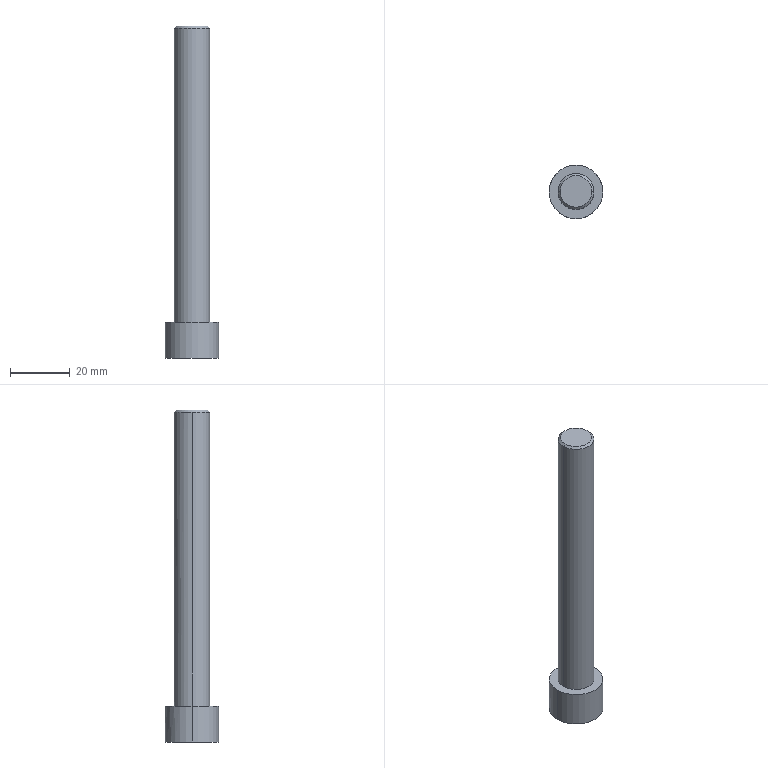Part | Creo | 1 solid | 16 faces | box 18 x 18 x 111 mm | volume 13555 mm3 | plane 10 | cylinder 4 | cone 2 | commonest cylinder face diameters 12 x2 18 x2
STEP:
#1=CARTESIAN_POINT('',(0.,0.,0.));
#2=DIRECTION('',(0.,0.,1.));
#3=DIRECTION('',(1.,0.,0.));
#4=AXIS2_PLACEMENT_3D('',#1,#2,#3);
#5=CARTESIAN_POINT('',(432.101,252.373,-117.152));
#6=VERTEX_POINT('',#5);
#7=CARTESIAN_POINT('',(420.101,252.373,-117.152));
#8=VERTEX_POINT('',#7);
#9=CARTESIAN_POINT('',(426.101,252.373,-117.152));
#10=DIRECTION('',(0.,0.,1.));
#11=DIRECTION('',(1.,0.,0.));
#12=AXIS2_PLACEMENT_3D('',#9,#10,#11);
#13=CIRCLE('',#12,6.);
#14=EDGE_CURVE('',#6,#8,#13,.T.);
#15=ORIENTED_EDGE('',*,*,#14,.T.);
#16=CARTESIAN_POINT('',(420.101,252.373,-215.441));
#17=VERTEX_POINT('',#16);
#18=CARTESIAN_POINT('',(420.101,252.373,-215.441));
#19=DIRECTION('',(0.,0.,1.));
#20=VECTOR('',#19,98.29);
#21=LINE('',#18,#20);
#22=EDGE_CURVE('',#17,#8,#21,.T.);
#23=ORIENTED_EDGE('',*,*,#22,.F.);
#24=CARTESIAN_POINT('',(426.101,258.373,-215.441));
#25=VERTEX_POINT('',#24);
#26=CARTESIAN_POINT('',(426.101,252.373,-215.441));
#27=DIRECTION('',(0.,0.,-1.));
#28=DIRECTION('',(-1.,0.,0.));
#29=AXIS2_PLACEMENT_3D('',#26,#27,#28);
#30=CIRCLE('',#29,6.);
#31=EDGE_CURVE('',#17,#25,#30,.T.);
#32=ORIENTED_EDGE('',*,*,#31,.T.);
#33=CARTESIAN_POINT('',(432.101,252.373,-215.441));
#34=VERTEX_POINT('',#33);
#35=CARTESIAN_POINT('',(426.101,252.373,-215.441));
#36=DIRECTION('',(0.,0.,-1.));
#37=DIRECTION('',(0.,1.,0.));
#38=AXIS2_PLACEMENT_3D('',#35,#36,#37);
#39=CIRCLE('',#38,6.);
#40=EDGE_CURVE('',#25,#34,#39,.T.);
#41=ORIENTED_EDGE('',*,*,#40,.T.);
#42=CARTESIAN_POINT('',(432.101,252.373,-215.441));
#43=DIRECTION('',(0.,0.,1.));
#44=VECTOR('',#43,98.29);
#45=LINE('',#42,#44);
#46=EDGE_CURVE('',#34,#6,#45,.T.);
#47=ORIENTED_EDGE('',*,*,#46,.T.);
#48=EDGE_LOOP('',(#15,#23,#32,#41,#47));
#49=FACE_OUTER_BOUND('',#48,.F.);
#50=CARTESIAN_POINT('',(426.101,252.373,-215.441));
#51=DIRECTION('',(0.,0.,1.));
#52=DIRECTION('',(1.,0.,0.));
#53=AXIS2_PLACEMENT_3D('',#50,#51,#52);
#54=CYLINDRICAL_SURFACE('',#53,6.);
#55=ADVANCED_FACE('',(#49),#54,.T.);
#56=CARTESIAN_POINT('',(426.101,257.662,-116.441));
#57=VERTEX_POINT('',#56);
#58=CARTESIAN_POINT('',(420.811,252.373,-116.441));
#59=VERTEX_POINT('',#58);
#60=CARTESIAN_POINT('',(426.101,252.373,-116.441));
#61=DIRECTION('',(0.,0.,1.));
#62=DIRECTION('',(0.,1.,0.));
#63=AXIS2_PLACEMENT_3D('',#60,#61,#62);
#64=CIRCLE('',#63,5.29);
#65=EDGE_CURVE('',#57,#59,#64,.T.);
#66=ORIENTED_EDGE('',*,*,#65,.T.);
#67=CARTESIAN_POINT('',(420.811,252.373,-116.441));
#68=DIRECTION('',(-0.7071,0.,-0.7071));
#69=VECTOR('',#68,1.005);
#70=LINE('',#67,#69);
#71=EDGE_CURVE('',#59,#8,#70,.T.);
#72=ORIENTED_EDGE('',*,*,#71,.T.);
#73=ORIENTED_EDGE('',*,*,#14,.F.);
#74=CARTESIAN_POINT('',(431.39,252.373,-116.441));
#75=VERTEX_POINT('',#74);
#76=CARTESIAN_POINT('',(431.39,252.373,-116.441));
#77=DIRECTION('',(0.7071,0.,-0.7071));
#78=VECTOR('',#77,1.005);
#79=LINE('',#76,#78);
#80=EDGE_CURVE('',#75,#6,#79,.T.);
#81=ORIENTED_EDGE('',*,*,#80,.F.);
#82=CARTESIAN_POINT('',(426.101,252.373,-116.441));
#83=DIRECTION('',(0.,0.,1.));
#84=DIRECTION('',(1.,0.,0.));
#85=AXIS2_PLACEMENT_3D('',#82,#83,#84);
#86=CIRCLE('',#85,5.29);
#87=EDGE_CURVE('',#75,#57,#86,.T.);
#88=ORIENTED_EDGE('',*,*,#87,.T.);
#89=EDGE_LOOP('',(#66,#72,#73,#81,#88));
#90=FACE_OUTER_BOUND('',#89,.F.);
#91=CARTESIAN_POINT('',(426.101,252.373,-116.797));
#92=DIRECTION('',(0.,0.,-1.));
#93=DIRECTION('',(-1.,0.,0.));
#94=AXIS2_PLACEMENT_3D('',#91,#92,#93);
#95=CONICAL_SURFACE('',#94,5.645,45.);
#96=ADVANCED_FACE('',(#90),#95,.T.);
#97=CARTESIAN_POINT('',(426.101,247.083,-116.441));
#98=VERTEX_POINT('',#97);
#99=CARTESIAN_POINT('',(426.101,252.373,-116.441));
#100=DIRECTION('',(0.,0.,1.));
#101=DIRECTION('',(0.,-1.,0.));
#102=AXIS2_PLACEMENT_3D('',#99,#100,#101);
#103=CIRCLE('',#102,5.29);
#104=EDGE_CURVE('',#98,#75,#103,.T.);
#105=ORIENTED_EDGE('',*,*,#104,.F.);
#106=CARTESIAN_POINT('',(426.101,252.373,-116.441));
#107=DIRECTION('',(0.,0.,1.));
#108=DIRECTION('',(-1.,0.,0.));
#109=AXIS2_PLACEMENT_3D('',#106,#107,#108);
#110=CIRCLE('',#109,5.29);
#111=EDGE_CURVE('',#59,#98,#110,.T.);
#112=ORIENTED_EDGE('',*,*,#111,.F.);
#113=ORIENTED_EDGE('',*,*,#65,.F.);
#114=ORIENTED_EDGE('',*,*,#87,.F.);
#115=EDGE_LOOP('',(#105,#112,#113,#114));
#116=FACE_OUTER_BOUND('',#115,.F.);
#117=CARTESIAN_POINT('',(426.101,252.373,-116.441));
#118=DIRECTION('',(0.,0.,-1.));
#119=DIRECTION('',(-1.,0.,0.));
#120=AXIS2_PLACEMENT_3D('',#117,#118,#119);
#121=PLANE('',#120);
#122=ADVANCED_FACE('',(#116),#121,.F.);
#123=ORIENTED_EDGE('',*,*,#111,.T.);
#124=ORIENTED_EDGE('',*,*,#104,.T.);
#125=ORIENTED_EDGE('',*,*,#80,.T.);
#126=CARTESIAN_POINT('',(426.101,246.373,-117.152));
#127=VERTEX_POINT('',#126);
#128=CARTESIAN_POINT('',(426.101,252.373,-117.152));
#129=DIRECTION('',(0.,0.,1.));
#130=DIRECTION('',(0.,-1.,0.));
#131=AXIS2_PLACEMENT_3D('',#128,#129,#130);
#132=CIRCLE('',#131,6.);
#133=EDGE_CURVE('',#127,#6,#132,.T.);
#134=ORIENTED_EDGE('',*,*,#133,.F.);
#135=CARTESIAN_POINT('',(426.101,252.373,-117.152));
#136=DIRECTION('',(0.,0.,1.));
#137=DIRECTION('',(-1.,0.,0.));
#138=AXIS2_PLACEMENT_3D('',#135,#136,#137);
#139=CIRCLE('',#138,6.);
#140=EDGE_CURVE('',#8,#127,#139,.T.);
#141=ORIENTED_EDGE('',*,*,#140,.F.);
#142=ORIENTED_EDGE('',*,*,#71,.F.);
#143=EDGE_LOOP('',(#123,#124,#125,#134,#141,#142));
#144=FACE_OUTER_BOUND('',#143,.F.);
#145=CARTESIAN_POINT('',(426.101,252.373,-116.797));
#146=DIRECTION('',(0.,0.,-1.));
#147=DIRECTION('',(-1.,0.,0.));
#148=AXIS2_PLACEMENT_3D('',#145,#146,#147);
#149=CONICAL_SURFACE('',#148,5.645,45.);
#150=ADVANCED_FACE('',(#144),#149,.T.);
#151=ORIENTED_EDGE('',*,*,#140,.T.);
#152=ORIENTED_EDGE('',*,*,#133,.T.);
#153=ORIENTED_EDGE('',*,*,#46,.F.);
#154=CARTESIAN_POINT('',(426.101,246.373,-215.441));
#155=VERTEX_POINT('',#154);
#156=CARTESIAN_POINT('',(426.101,252.373,-215.441));
#157=DIRECTION('',(0.,0.,-1.));
#158=DIRECTION('',(1.,0.,0.));
#159=AXIS2_PLACEMENT_3D('',#156,#157,#158);
#160=CIRCLE('',#159,6.);
#161=EDGE_CURVE('',#34,#155,#160,.T.);
#162=ORIENTED_EDGE('',*,*,#161,.T.);
#163=CARTESIAN_POINT('',(426.101,252.373,-215.441));
#164=DIRECTION('',(0.,0.,-1.));
#165=DIRECTION('',(0.,-1.,0.));
#166=AXIS2_PLACEMENT_3D('',#163,#164,#165);
#167=CIRCLE('',#166,6.);
#168=EDGE_CURVE('',#155,#17,#167,.T.);
#169=ORIENTED_EDGE('',*,*,#168,.T.);
#170=ORIENTED_EDGE('',*,*,#22,.T.);
#171=EDGE_LOOP('',(#151,#152,#153,#162,#169,#170));
#172=FACE_OUTER_BOUND('',#171,.F.);
#173=CARTESIAN_POINT('',(426.101,252.373,-215.441));
#174=DIRECTION('',(0.,0.,1.));
#175=DIRECTION('',(1.,0.,0.));
#176=AXIS2_PLACEMENT_3D('',#173,#174,#175);
#177=CYLINDRICAL_SURFACE('',#176,6.);
#178=ADVANCED_FACE('',(#172),#177,.T.);
#179=CARTESIAN_POINT('',(426.101,243.373,-215.441));
#180=VERTEX_POINT('',#179);
#181=CARTESIAN_POINT('',(435.101,252.373,-215.441));
#182=VERTEX_POINT('',#181);
#183=CARTESIAN_POINT('',(426.101,252.373,-215.441));
#184=DIRECTION('',(0.,0.,1.));
#185=DIRECTION('',(0.,-1.,0.));
#186=AXIS2_PLACEMENT_3D('',#183,#184,#185);
#187=CIRCLE('',#186,9.);
#188=EDGE_CURVE('',#180,#182,#187,.T.);
#189=ORIENTED_EDGE('',*,*,#188,.F.);
#190=CARTESIAN_POINT('',(417.101,252.373,-215.441));
#191=VERTEX_POINT('',#190);
#192=CARTESIAN_POINT('',(426.101,252.373,-215.441));
#193=DIRECTION('',(0.,0.,1.));
#194=DIRECTION('',(-1.,0.,0.));
#195=AXIS2_PLACEMENT_3D('',#192,#193,#194);
#196=CIRCLE('',#195,9.);
#197=EDGE_CURVE('',#191,#180,#196,.T.);
#198=ORIENTED_EDGE('',*,*,#197,.F.);
#199=CARTESIAN_POINT('',(426.101,252.373,-215.441));
#200=DIRECTION('',(0.,0.,1.));
#201=DIRECTION('',(1.,0.,0.));
#202=AXIS2_PLACEMENT_3D('',#199,#200,#201);
#203=CIRCLE('',#202,9.);
#204=EDGE_CURVE('',#182,#191,#203,.T.);
#205=ORIENTED_EDGE('',*,*,#204,.F.);
#206=EDGE_LOOP('',(#189,#198,#205));
#207=FACE_OUTER_BOUND('',#206,.F.);
#208=ORIENTED_EDGE('',*,*,#168,.F.);
#209=ORIENTED_EDGE('',*,*,#161,.F.);
#210=ORIENTED_EDGE('',*,*,#40,.F.);
#211=ORIENTED_EDGE('',*,*,#31,.F.);
#212=EDGE_LOOP('',(#208,#209,#210,#211));
#213=FACE_BOUND('',#212,.F.);
#214=CARTESIAN_POINT('',(426.101,252.373,-215.441));
#215=DIRECTION('',(0.,0.,1.));
#216=DIRECTION('',(1.,0.,0.));
#217=AXIS2_PLACEMENT_3D('',#214,#215,#216);
#218=PLANE('',#217);
#219=ADVANCED_FACE('',(#207,#213),#218,.T.);
#220=CARTESIAN_POINT('',(435.101,252.373,-227.441));
#221=VERTEX_POINT('',#220);
#222=CARTESIAN_POINT('',(426.101,243.373,-227.441));
#223=VERTEX_POINT('',#222);
#224=CARTESIAN_POINT('',(426.101,252.373,-227.441));
#225=DIRECTION('',(0.,0.,-1.));
#226=DIRECTION('',(1.,0.,0.));
#227=AXIS2_PLACEMENT_3D('',#224,#225,#226);
#228=CIRCLE('',#227,9.);
#229=EDGE_CURVE('',#221,#223,#228,.T.);
#230=ORIENTED_EDGE('',*,*,#229,.T.);
#231=CARTESIAN_POINT('',(417.101,252.373,-227.441));
#232=VERTEX_POINT('',#231);
#233=CARTESIAN_POINT('',(426.101,252.373,-227.441));
#234=DIRECTION('',(0.,0.,-1.));
#235=DIRECTION('',(0.,-1.,0.));
#236=AXIS2_PLACEMENT_3D('',#233,#234,#235);
#237=CIRCLE('',#236,9.);
#238=EDGE_CURVE('',#223,#232,#237,.T.);
#239=ORIENTED_EDGE('',*,*,#238,.T.);
#240=CARTESIAN_POINT('',(417.101,252.373,-215.441));
#241=DIRECTION('',(0.,0.,-1.));
#242=VECTOR('',#241,12.);
#243=LINE('',#240,#242);
#244=EDGE_CURVE('',#191,#232,#243,.T.);
#245=ORIENTED_EDGE('',*,*,#244,.F.);
#246=ORIENTED_EDGE('',*,*,#197,.T.);
#247=ORIENTED_EDGE('',*,*,#188,.T.);
#248=CARTESIAN_POINT('',(435.101,252.373,-215.441));
#249=DIRECTION('',(0.,0.,-1.));
#250=VECTOR('',#249,12.);
#251=LINE('',#248,#250);
#252=EDGE_CURVE('',#182,#221,#251,.T.);
#253=ORIENTED_EDGE('',*,*,#252,.T.);
#254=EDGE_LOOP('',(#230,#239,#245,#246,#247,#253));
#255=FACE_OUTER_BOUND('',#254,.F.);
#256=CARTESIAN_POINT('',(426.101,252.373,-215.441));
#257=DIRECTION('',(0.,0.,-1.));
#258=DIRECTION('',(-1.,0.,0.));
#259=AXIS2_PLACEMENT_3D('',#256,#257,#258);
#260=CYLINDRICAL_SURFACE('',#259,9.);
#261=ADVANCED_FACE('',(#255),#260,.T.);
#262=ORIENTED_EDGE('',*,*,#238,.F.);
#263=ORIENTED_EDGE('',*,*,#229,.F.);
#264=CARTESIAN_POINT('',(426.101,261.373,-227.441));
#265=VERTEX_POINT('',#264);
#266=CARTESIAN_POINT('',(426.101,252.373,-227.441));
#267=DIRECTION('',(0.,0.,-1.));
#268=DIRECTION('',(0.,1.,0.));
#269=AXIS2_PLACEMENT_3D('',#266,#267,#268);
#270=CIRCLE('',#269,9.);
#271=EDGE_CURVE('',#265,#221,#270,.T.);
#272=ORIENTED_EDGE('',*,*,#271,.F.);
#273=CARTESIAN_POINT('',(426.101,252.373,-227.441));
#274=DIRECTION('',(0.,0.,-1.));
#275=DIRECTION('',(-1.,0.,0.));
#276=AXIS2_PLACEMENT_3D('',#273,#274,#275);
#277=CIRCLE('',#276,9.);
#278=EDGE_CURVE('',#232,#265,#277,.T.);
#279=ORIENTED_EDGE('',*,*,#278,.F.);
#280=EDGE_LOOP('',(#262,#263,#272,#279));
#281=FACE_OUTER_BOUND('',#280,.F.);
#282=CARTESIAN_POINT('',(431.101,249.486,-227.441));
#283=VERTEX_POINT('',#282);
#284=CARTESIAN_POINT('',(431.101,255.259,-227.441));
#285=VERTEX_POINT('',#284);
#286=CARTESIAN_POINT('',(431.101,249.486,-227.441));
#287=DIRECTION('',(0.,1.,0.));
#288=VECTOR('',#287,5.774);
#289=LINE('',#286,#288);
#290=EDGE_CURVE('',#283,#285,#289,.T.);
#291=ORIENTED_EDGE('',*,*,#290,.F.);
#292=CARTESIAN_POINT('',(426.101,246.599,-227.441));
#293=VERTEX_POINT('',#292);
#294=CARTESIAN_POINT('',(426.101,246.599,-227.441));
#295=DIRECTION('',(0.866,0.5,0.));
#296=VECTOR('',#295,5.774);
#297=LINE('',#294,#296);
#298=EDGE_CURVE('',#293,#283,#297,.T.);
#299=ORIENTED_EDGE('',*,*,#298,.F.);
#300=CARTESIAN_POINT('',(421.101,249.486,-227.441));
#301=VERTEX_POINT('',#300);
#302=CARTESIAN_POINT('',(421.101,249.486,-227.441));
#303=DIRECTION('',(0.866,-0.5,0.));
#304=VECTOR('',#303,5.774);
#305=LINE('',#302,#304);
#306=EDGE_CURVE('',#301,#293,#305,.T.);
#307=ORIENTED_EDGE('',*,*,#306,.F.);
#308=CARTESIAN_POINT('',(421.101,255.259,-227.441));
#309=VERTEX_POINT('',#308);
#310=CARTESIAN_POINT('',(421.101,255.259,-227.441));
#311=DIRECTION('',(0.,-1.,0.));
#312=VECTOR('',#311,5.774);
#313=LINE('',#310,#312);
#314=EDGE_CURVE('',#309,#301,#313,.T.);
#315=ORIENTED_EDGE('',*,*,#314,.F.);
#316=CARTESIAN_POINT('',(426.101,258.146,-227.441));
#317=VERTEX_POINT('',#316);
#318=CARTESIAN_POINT('',(426.101,258.146,-227.441));
#319=DIRECTION('',(-0.866,-0.5,0.));
#320=VECTOR('',#319,5.774);
#321=LINE('',#318,#320);
#322=EDGE_CURVE('',#317,#309,#321,.T.);
#323=ORIENTED_EDGE('',*,*,#322,.F.);
#324=CARTESIAN_POINT('',(431.101,255.259,-227.441));
#325=DIRECTION('',(-0.866,0.5,0.));
#326=VECTOR('',#325,5.774);
#327=LINE('',#324,#326);
#328=EDGE_CURVE('',#285,#317,#327,.T.);
#329=ORIENTED_EDGE('',*,*,#328,.F.);
#330=EDGE_LOOP('',(#291,#299,#307,#315,#323,#329));
#331=FACE_BOUND('',#330,.F.);
#332=CARTESIAN_POINT('',(426.101,252.373,-227.441));
#333=DIRECTION('',(0.,0.,-1.));
#334=DIRECTION('',(-1.,0.,0.));
#335=AXIS2_PLACEMENT_3D('',#332,#333,#334);
#336=PLANE('',#335);
#337=ADVANCED_FACE('',(#281,#331),#336,.T.);
#338=ORIENTED_EDGE('',*,*,#290,.T.);
#339=CARTESIAN_POINT('',(431.101,255.259,-219.521));
#340=VERTEX_POINT('',#339);
#341=CARTESIAN_POINT('',(431.101,255.259,-227.441));
#342=DIRECTION('',(0.,0.,1.));
#343=VECTOR('',#342,7.92);
#344=LINE('',#341,#343);
#345=EDGE_CURVE('',#285,#340,#344,.T.);
#346=ORIENTED_EDGE('',*,*,#345,.T.);
#347=CARTESIAN_POINT('',(431.101,249.486,-219.521));
#348=VERTEX_POINT('',#347);
#349=CARTESIAN_POINT('',(431.101,249.486,-219.521));
#350=DIRECTION('',(0.,1.,0.));
#351=VECTOR('',#350,5.774);
#352=LINE('',#349,#351);
#353=EDGE_CURVE('',#348,#340,#352,.T.);
#354=ORIENTED_EDGE('',*,*,#353,.F.);
#355=CARTESIAN_POINT('',(431.101,249.486,-227.441));
#356=DIRECTION('',(0.,0.,1.));
#357=VECTOR('',#356,7.92);
#358=LINE('',#355,#357);
#359=EDGE_CURVE('',#283,#348,#358,.T.);
#360=ORIENTED_EDGE('',*,*,#359,.F.);
#361=EDGE_LOOP('',(#338,#346,#354,#360));
#362=FACE_OUTER_BOUND('',#361,.F.);
#363=CARTESIAN_POINT('',(431.101,255.259,-219.521));
#364=DIRECTION('',(1.,0.,0.));
#365=DIRECTION('',(0.,0.,-1.));
#366=AXIS2_PLACEMENT_3D('',#363,#364,#365);
#367=PLANE('',#366);
#368=ADVANCED_FACE('',(#362),#367,.F.);
#369=ORIENTED_EDGE('',*,*,#328,.T.);
#370=CARTESIAN_POINT('',(426.101,258.146,-219.521));
#371=VERTEX_POINT('',#370);
#372=CARTESIAN_POINT('',(426.101,258.146,-227.441));
#373=DIRECTION('',(0.,0.,1.));
#374=VECTOR('',#373,7.92);
#375=LINE('',#372,#374);
#376=EDGE_CURVE('',#317,#371,#375,.T.);
#377=ORIENTED_EDGE('',*,*,#376,.T.);
#378=CARTESIAN_POINT('',(426.101,258.146,-219.521));
#379=DIRECTION('',(0.866,-0.5,0.));
#380=VECTOR('',#379,5.774);
#381=LINE('',#378,#380);
#382=EDGE_CURVE('',#371,#340,#381,.T.);
#383=ORIENTED_EDGE('',*,*,#382,.T.);
#384=ORIENTED_EDGE('',*,*,#345,.F.);
#385=EDGE_LOOP('',(#369,#377,#383,#384));
#386=FACE_OUTER_BOUND('',#385,.F.);
#387=CARTESIAN_POINT('',(426.101,258.146,-219.521));
#388=DIRECTION('',(0.5,0.866,0.));
#389=DIRECTION('',(-0.866,0.5,0.));
#390=AXIS2_PLACEMENT_3D('',#387,#388,#389);
#391=PLANE('',#390);
#392=ADVANCED_FACE('',(#386),#391,.F.);
#393=ORIENTED_EDGE('',*,*,#322,.T.);
#394=CARTESIAN_POINT('',(421.101,255.259,-219.521));
#395=VERTEX_POINT('',#394);
#396=CARTESIAN_POINT('',(421.101,255.259,-227.441));
#397=DIRECTION('',(0.,0.,1.));
#398=VECTOR('',#397,7.92);
#399=LINE('',#396,#398);
#400=EDGE_CURVE('',#309,#395,#399,.T.);
#401=ORIENTED_EDGE('',*,*,#400,.T.);
#402=CARTESIAN_POINT('',(421.101,255.259,-219.521));
#403=DIRECTION('',(0.866,0.5,0.));
#404=VECTOR('',#403,5.774);
#405=LINE('',#402,#404);
#406=EDGE_CURVE('',#395,#371,#405,.T.);
#407=ORIENTED_EDGE('',*,*,#406,.T.);
#408=ORIENTED_EDGE('',*,*,#376,.F.);
#409=EDGE_LOOP('',(#393,#401,#407,#408));
#410=FACE_OUTER_BOUND('',#409,.F.);
#411=CARTESIAN_POINT('',(421.101,255.259,-219.521));
#412=DIRECTION('',(-0.5,0.866,0.));
#413=DIRECTION('',(-0.866,-0.5,0.));
#414=AXIS2_PLACEMENT_3D('',#411,#412,#413);
#415=PLANE('',#414);
#416=ADVANCED_FACE('',(#410),#415,.F.);
#417=ORIENTED_EDGE('',*,*,#314,.T.);
#418=CARTESIAN_POINT('',(421.101,249.486,-219.521));
#419=VERTEX_POINT('',#418);
#420=CARTESIAN_POINT('',(421.101,249.486,-227.441));
#421=DIRECTION('',(0.,0.,1.));
#422=VECTOR('',#421,7.92);
#423=LINE('',#420,#422);
#424=EDGE_CURVE('',#301,#419,#423,.T.);
#425=ORIENTED_EDGE('',*,*,#424,.T.);
#426=CARTESIAN_POINT('',(421.101,255.259,-219.521));
#427=DIRECTION('',(0.,-1.,0.));
#428=VECTOR('',#427,5.774);
#429=LINE('',#426,#428);
#430=EDGE_CURVE('',#395,#419,#429,.T.);
#431=ORIENTED_EDGE('',*,*,#430,.F.);
#432=ORIENTED_EDGE('',*,*,#400,.F.);
#433=EDGE_LOOP('',(#417,#425,#431,#432));
#434=FACE_OUTER_BOUND('',#433,.F.);
#435=CARTESIAN_POINT('',(421.101,249.486,-219.521));
#436=DIRECTION('',(-1.,0.,0.));
#437=DIRECTION('',(0.,0.,1.));
#438=AXIS2_PLACEMENT_3D('',#435,#436,#437);
#439=PLANE('',#438);
#440=ADVANCED_FACE('',(#434),#439,.F.);
#441=ORIENTED_EDGE('',*,*,#306,.T.);
#442=CARTESIAN_POINT('',(426.101,246.599,-219.521));
#443=VERTEX_POINT('',#442);
#444=CARTESIAN_POINT('',(426.101,246.599,-227.441));
#445=DIRECTION('',(0.,0.,1.));
#446=VECTOR('',#445,7.92);
#447=LINE('',#444,#446);
#448=EDGE_CURVE('',#293,#443,#447,.T.);
#449=ORIENTED_EDGE('',*,*,#448,.T.);
#450=CARTESIAN_POINT('',(426.101,246.599,-219.521));
#451=DIRECTION('',(-0.866,0.5,0.));
#452=VECTOR('',#451,5.774);
#453=LINE('',#450,#452);
#454=EDGE_CURVE('',#443,#419,#453,.T.);
#455=ORIENTED_EDGE('',*,*,#454,.T.);
#456=ORIENTED_EDGE('',*,*,#424,.F.);
#457=EDGE_LOOP('',(#441,#449,#455,#456));
#458=FACE_OUTER_BOUND('',#457,.F.);
#459=CARTESIAN_POINT('',(426.101,246.599,-219.521));
#460=DIRECTION('',(-0.5,-0.866,0.));
#461=DIRECTION('',(0.866,-0.5,0.));
#462=AXIS2_PLACEMENT_3D('',#459,#460,#461);
#463=PLANE('',#462);
#464=ADVANCED_FACE('',(#458),#463,.F.);
#465=ORIENTED_EDGE('',*,*,#298,.T.);
#466=ORIENTED_EDGE('',*,*,#359,.T.);
#467=CARTESIAN_POINT('',(431.101,249.486,-219.521));
#468=DIRECTION('',(-0.866,-0.5,0.));
#469=VECTOR('',#468,5.774);
#470=LINE('',#467,#469);
#471=EDGE_CURVE('',#348,#443,#470,.T.);
#472=ORIENTED_EDGE('',*,*,#471,.T.);
#473=ORIENTED_EDGE('',*,*,#448,.F.);
#474=EDGE_LOOP('',(#465,#466,#472,#473));
#475=FACE_OUTER_BOUND('',#474,.F.);
#476=CARTESIAN_POINT('',(431.101,249.486,-219.521));
#477=DIRECTION('',(0.5,-0.866,0.));
#478=DIRECTION('',(0.866,0.5,0.));
#479=AXIS2_PLACEMENT_3D('',#476,#477,#478);
#480=PLANE('',#479);
#481=ADVANCED_FACE('',(#475),#480,.F.);
#482=ORIENTED_EDGE('',*,*,#353,.T.);
#483=ORIENTED_EDGE('',*,*,#382,.F.);
#484=ORIENTED_EDGE('',*,*,#406,.F.);
#485=ORIENTED_EDGE('',*,*,#430,.T.);
#486=ORIENTED_EDGE('',*,*,#454,.F.);
#487=ORIENTED_EDGE('',*,*,#471,.F.);
#488=EDGE_LOOP('',(#482,#483,#484,#485,#486,#487));
#489=FACE_OUTER_BOUND('',#488,.F.);
#490=CARTESIAN_POINT('',(431.101,249.486,-219.521));
#491=DIRECTION('',(0.,0.,-1.));
#492=DIRECTION('',(-1.,0.,0.));
#493=AXIS2_PLACEMENT_3D('',#490,#491,#492);
#494=PLANE('',#493);
#495=ADVANCED_FACE('',(#489),#494,.T.);
#496=ORIENTED_EDGE('',*,*,#271,.T.);
#497=ORIENTED_EDGE('',*,*,#252,.F.);
#498=ORIENTED_EDGE('',*,*,#204,.T.);
#499=ORIENTED_EDGE('',*,*,#244,.T.);
#500=ORIENTED_EDGE('',*,*,#278,.T.);
#501=EDGE_LOOP('',(#496,#497,#498,#499,#500));
#502=FACE_OUTER_BOUND('',#501,.F.);
#503=CARTESIAN_POINT('',(426.101,252.373,-215.441));
#504=DIRECTION('',(0.,0.,-1.));
#505=DIRECTION('',(-1.,0.,0.));
#506=AXIS2_PLACEMENT_3D('',#503,#504,#505);
#507=CYLINDRICAL_SURFACE('',#506,9.);
#508=ADVANCED_FACE('',(#502),#507,.T.);
#509=CLOSED_SHELL('',(#55,#96,#122,#150,#178,#219,#261,#337,#368,#392,#416,#440,#464,#481,#495,#508));
#510=MANIFOLD_SOLID_BREP('',#509);
#511=(LENGTH_UNIT()NAMED_UNIT(*)SI_UNIT(.MILLI.,.METRE.));
#512=UNCERTAINTY_MEASURE_WITH_UNIT(LENGTH_MEASURE(0.01139),#511,'','');
#513=(NAMED_UNIT(*)PLANE_ANGLE_UNIT()SI_UNIT($,.RADIAN.));
#514=PLANE_ANGLE_MEASURE_WITH_UNIT(PLANE_ANGLE_MEASURE(0.01745),#513);
#515=(CONVERSION_BASED_UNIT('DEGREE',#514)NAMED_UNIT(*)PLANE_ANGLE_UNIT());
#516=(NAMED_UNIT(*)SI_UNIT($,.STERADIAN.)SOLID_ANGLE_UNIT());
#517=(GEOMETRIC_REPRESENTATION_CONTEXT(3)GLOBAL_UNCERTAINTY_ASSIGNED_CONTEXT((#512))GLOBAL_UNIT_ASSIGNED_CONTEXT((#511,#515,#516))REPRESENTATION_CONTEXT('',''));
#518=ADVANCED_BREP_SHAPE_REPRESENTATION('',(#4,#510),#517);